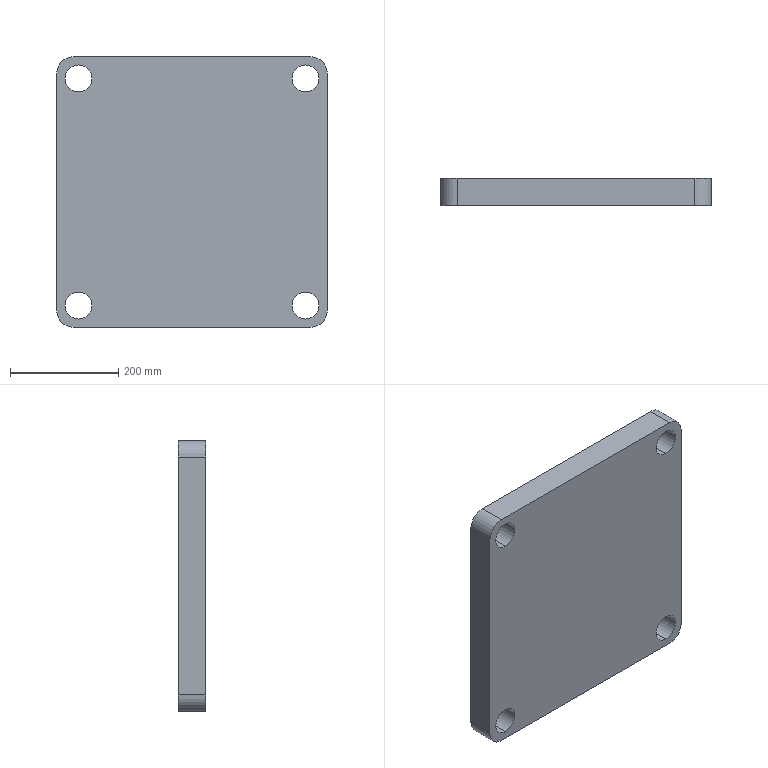Part | SolidWorks | features ICE 2, Extrusion 1 | 1 solid | 27 faces | box 500 x 50 x 500 mm | volume 6892126 mm3 | cylinder 16 | plane 11 | commonest cylinder face diameters 50 x8 60 x4 70 x4
STEP:
#1=CARTESIAN_POINT('',(-210.,0.,185.));
#2=VERTEX_POINT('',#1);
#3=CARTESIAN_POINT('',(-210.,0.,235.));
#4=VERTEX_POINT('',#3);
#5=CARTESIAN_POINT('',(-210.,0.,210.));
#6=DIRECTION('',(0.,1.,0.));
#7=DIRECTION('',(0.,0.,-1.));
#8=AXIS2_PLACEMENT_3D('',#5,#6,#7);
#9=CIRCLE('',#8,25.);
#10=EDGE_CURVE('',#2,#4,#9,.T.);
#11=ORIENTED_EDGE('',*,*,#10,.F.);
#12=CARTESIAN_POINT('',(-210.,50.,185.));
#13=VERTEX_POINT('',#12);
#14=CARTESIAN_POINT('',(-210.,-0.001,185.));
#15=DIRECTION('',(0.,1.,0.));
#16=VECTOR('',#15,1000.);
#17=LINE('',#14,#16);
#18=EDGE_CURVE('',#2,#13,#17,.T.);
#19=ORIENTED_EDGE('',*,*,#18,.T.);
#20=CARTESIAN_POINT('',(-210.,50.,235.));
#21=VERTEX_POINT('',#20);
#22=CARTESIAN_POINT('',(-210.,50.,210.));
#23=DIRECTION('',(0.,1.,0.));
#24=DIRECTION('',(0.,0.,-1.));
#25=AXIS2_PLACEMENT_3D('',#22,#23,#24);
#26=CIRCLE('',#25,25.);
#27=EDGE_CURVE('',#13,#21,#26,.T.);
#28=ORIENTED_EDGE('',*,*,#27,.T.);
#29=CARTESIAN_POINT('',(-210.,-0.001,235.));
#30=DIRECTION('',(0.,1.,0.));
#31=VECTOR('',#30,1000.);
#32=LINE('',#29,#31);
#33=EDGE_CURVE('',#4,#21,#32,.T.);
#34=ORIENTED_EDGE('',*,*,#33,.F.);
#35=EDGE_LOOP('',(#11,#19,#28,#34));
#36=FACE_OUTER_BOUND('',#35,.T.);
#37=CARTESIAN_POINT('',(-210.,-0.001,210.));
#38=DIRECTION('',(0.,1.,0.));
#39=DIRECTION('',(0.,0.,1.));
#40=AXIS2_PLACEMENT_3D('',#37,#38,#39);
#41=CYLINDRICAL_SURFACE('',#40,25.);
#42=ADVANCED_FACE('',(#36),#41,.F.);
#43=CARTESIAN_POINT('',(210.,0.,185.));
#44=VERTEX_POINT('',#43);
#45=CARTESIAN_POINT('',(210.,0.,235.));
#46=VERTEX_POINT('',#45);
#47=CARTESIAN_POINT('',(210.,0.,210.));
#48=DIRECTION('',(0.,1.,0.));
#49=DIRECTION('',(0.,0.,-1.));
#50=AXIS2_PLACEMENT_3D('',#47,#48,#49);
#51=CIRCLE('',#50,25.);
#52=EDGE_CURVE('',#44,#46,#51,.T.);
#53=ORIENTED_EDGE('',*,*,#52,.F.);
#54=CARTESIAN_POINT('',(210.,50.,185.));
#55=VERTEX_POINT('',#54);
#56=CARTESIAN_POINT('',(210.,-0.001,185.));
#57=DIRECTION('',(0.,1.,0.));
#58=VECTOR('',#57,1000.);
#59=LINE('',#56,#58);
#60=EDGE_CURVE('',#44,#55,#59,.T.);
#61=ORIENTED_EDGE('',*,*,#60,.T.);
#62=CARTESIAN_POINT('',(210.,50.,235.));
#63=VERTEX_POINT('',#62);
#64=CARTESIAN_POINT('',(210.,50.,210.));
#65=DIRECTION('',(0.,1.,0.));
#66=DIRECTION('',(0.,0.,1.));
#67=AXIS2_PLACEMENT_3D('',#64,#65,#66);
#68=CIRCLE('',#67,25.);
#69=EDGE_CURVE('',#55,#63,#68,.T.);
#70=ORIENTED_EDGE('',*,*,#69,.T.);
#71=CARTESIAN_POINT('',(210.,-0.001,235.));
#72=DIRECTION('',(0.,1.,0.));
#73=VECTOR('',#72,1000.);
#74=LINE('',#71,#73);
#75=EDGE_CURVE('',#46,#63,#74,.T.);
#76=ORIENTED_EDGE('',*,*,#75,.F.);
#77=EDGE_LOOP('',(#53,#61,#70,#76));
#78=FACE_OUTER_BOUND('',#77,.T.);
#79=CARTESIAN_POINT('',(210.,-0.001,210.));
#80=DIRECTION('',(0.,1.,0.));
#81=DIRECTION('',(0.,0.,1.));
#82=AXIS2_PLACEMENT_3D('',#79,#80,#81);
#83=CYLINDRICAL_SURFACE('',#82,25.);
#84=ADVANCED_FACE('',(#78),#83,.F.);
#85=CARTESIAN_POINT('',(210.,0.,-235.));
#86=VERTEX_POINT('',#85);
#87=CARTESIAN_POINT('',(210.,0.,-185.));
#88=VERTEX_POINT('',#87);
#89=CARTESIAN_POINT('',(210.,0.,-210.));
#90=DIRECTION('',(0.,1.,0.));
#91=DIRECTION('',(0.,0.,-1.));
#92=AXIS2_PLACEMENT_3D('',#89,#90,#91);
#93=CIRCLE('',#92,25.);
#94=EDGE_CURVE('',#86,#88,#93,.T.);
#95=ORIENTED_EDGE('',*,*,#94,.F.);
#96=CARTESIAN_POINT('',(210.,50.,-235.));
#97=VERTEX_POINT('',#96);
#98=CARTESIAN_POINT('',(210.,-0.001,-235.));
#99=DIRECTION('',(0.,1.,0.));
#100=VECTOR('',#99,1000.);
#101=LINE('',#98,#100);
#102=EDGE_CURVE('',#86,#97,#101,.T.);
#103=ORIENTED_EDGE('',*,*,#102,.T.);
#104=CARTESIAN_POINT('',(210.,50.,-185.));
#105=VERTEX_POINT('',#104);
#106=CARTESIAN_POINT('',(210.,50.,-210.));
#107=DIRECTION('',(0.,1.,0.));
#108=DIRECTION('',(0.,0.,-1.));
#109=AXIS2_PLACEMENT_3D('',#106,#107,#108);
#110=CIRCLE('',#109,25.);
#111=EDGE_CURVE('',#97,#105,#110,.T.);
#112=ORIENTED_EDGE('',*,*,#111,.T.);
#113=CARTESIAN_POINT('',(210.,-0.001,-185.));
#114=DIRECTION('',(0.,1.,0.));
#115=VECTOR('',#114,1000.);
#116=LINE('',#113,#115);
#117=EDGE_CURVE('',#88,#105,#116,.T.);
#118=ORIENTED_EDGE('',*,*,#117,.F.);
#119=EDGE_LOOP('',(#95,#103,#112,#118));
#120=FACE_OUTER_BOUND('',#119,.T.);
#121=CARTESIAN_POINT('',(210.,-0.001,-210.));
#122=DIRECTION('',(0.,1.,0.));
#123=DIRECTION('',(0.,0.,1.));
#124=AXIS2_PLACEMENT_3D('',#121,#122,#123);
#125=CYLINDRICAL_SURFACE('',#124,25.);
#126=ADVANCED_FACE('',(#120),#125,.F.);
#127=CARTESIAN_POINT('',(-210.,0.,-235.));
#128=VERTEX_POINT('',#127);
#129=CARTESIAN_POINT('',(-210.,0.,-185.));
#130=VERTEX_POINT('',#129);
#131=CARTESIAN_POINT('',(-210.,0.,-210.));
#132=DIRECTION('',(0.,1.,0.));
#133=DIRECTION('',(0.,0.,-1.));
#134=AXIS2_PLACEMENT_3D('',#131,#132,#133);
#135=CIRCLE('',#134,25.);
#136=EDGE_CURVE('',#128,#130,#135,.T.);
#137=ORIENTED_EDGE('',*,*,#136,.F.);
#138=CARTESIAN_POINT('',(-210.,50.,-235.));
#139=VERTEX_POINT('',#138);
#140=CARTESIAN_POINT('',(-210.,-0.001,-235.));
#141=DIRECTION('',(0.,1.,0.));
#142=VECTOR('',#141,1000.);
#143=LINE('',#140,#142);
#144=EDGE_CURVE('',#128,#139,#143,.T.);
#145=ORIENTED_EDGE('',*,*,#144,.T.);
#146=CARTESIAN_POINT('',(-210.,50.,-185.));
#147=VERTEX_POINT('',#146);
#148=CARTESIAN_POINT('',(-210.,50.,-210.));
#149=DIRECTION('',(0.,1.,0.));
#150=DIRECTION('',(0.,0.,1.));
#151=AXIS2_PLACEMENT_3D('',#148,#149,#150);
#152=CIRCLE('',#151,25.);
#153=EDGE_CURVE('',#139,#147,#152,.T.);
#154=ORIENTED_EDGE('',*,*,#153,.T.);
#155=CARTESIAN_POINT('',(-210.,-0.001,-185.));
#156=DIRECTION('',(0.,1.,0.));
#157=VECTOR('',#156,1000.);
#158=LINE('',#155,#157);
#159=EDGE_CURVE('',#130,#147,#158,.T.);
#160=ORIENTED_EDGE('',*,*,#159,.F.);
#161=EDGE_LOOP('',(#137,#145,#154,#160));
#162=FACE_OUTER_BOUND('',#161,.T.);
#163=CARTESIAN_POINT('',(-210.,-0.001,-210.));
#164=DIRECTION('',(0.,1.,0.));
#165=DIRECTION('',(0.,0.,1.));
#166=AXIS2_PLACEMENT_3D('',#163,#164,#165);
#167=CYLINDRICAL_SURFACE('',#166,25.);
#168=ADVANCED_FACE('',(#162),#167,.F.);
#169=CARTESIAN_POINT('',(-250.,0.,220.));
#170=VERTEX_POINT('',#169);
#171=CARTESIAN_POINT('',(-220.,0.,250.));
#172=VERTEX_POINT('',#171);
#173=CARTESIAN_POINT('',(-220.,0.,220.));
#174=DIRECTION('',(0.,1.,0.));
#175=DIRECTION('',(0.,0.,-1.));
#176=AXIS2_PLACEMENT_3D('',#173,#174,#175);
#177=CIRCLE('',#176,30.);
#178=EDGE_CURVE('',#170,#172,#177,.T.);
#179=ORIENTED_EDGE('',*,*,#178,.T.);
#180=CARTESIAN_POINT('',(-220.,50.,250.));
#181=VERTEX_POINT('',#180);
#182=CARTESIAN_POINT('',(-220.,50.,250.));
#183=DIRECTION('',(0.,-1.,0.));
#184=VECTOR('',#183,1000.);
#185=LINE('',#182,#184);
#186=EDGE_CURVE('',#181,#172,#185,.T.);
#187=ORIENTED_EDGE('',*,*,#186,.F.);
#188=CARTESIAN_POINT('',(-250.,50.,220.));
#189=VERTEX_POINT('',#188);
#190=CARTESIAN_POINT('',(-220.,50.,220.));
#191=DIRECTION('',(0.,1.,0.));
#192=DIRECTION('',(0.,0.,-1.));
#193=AXIS2_PLACEMENT_3D('',#190,#191,#192);
#194=CIRCLE('',#193,30.);
#195=EDGE_CURVE('',#189,#181,#194,.T.);
#196=ORIENTED_EDGE('',*,*,#195,.F.);
#197=CARTESIAN_POINT('',(-250.,50.,220.));
#198=DIRECTION('',(0.,-1.,0.));
#199=VECTOR('',#198,1000.);
#200=LINE('',#197,#199);
#201=EDGE_CURVE('',#189,#170,#200,.T.);
#202=ORIENTED_EDGE('',*,*,#201,.T.);
#203=EDGE_LOOP('',(#179,#187,#196,#202));
#204=FACE_OUTER_BOUND('',#203,.T.);
#205=CARTESIAN_POINT('',(-220.,50.,220.));
#206=DIRECTION('',(0.,-1.,0.));
#207=DIRECTION('',(0.,0.,-1.));
#208=AXIS2_PLACEMENT_3D('',#205,#206,#207);
#209=CYLINDRICAL_SURFACE('',#208,30.);
#210=ADVANCED_FACE('',(#204),#209,.T.);
#211=CARTESIAN_POINT('',(220.,0.,250.));
#212=VERTEX_POINT('',#211);
#213=CARTESIAN_POINT('',(-220.,0.,250.));
#214=DIRECTION('',(1.,0.,0.));
#215=VECTOR('',#214,1000.);
#216=LINE('',#213,#215);
#217=EDGE_CURVE('',#172,#212,#216,.T.);
#218=ORIENTED_EDGE('',*,*,#217,.T.);
#219=CARTESIAN_POINT('',(220.,50.,250.));
#220=VERTEX_POINT('',#219);
#221=CARTESIAN_POINT('',(220.,50.,250.));
#222=DIRECTION('',(0.,-1.,0.));
#223=VECTOR('',#222,1000.);
#224=LINE('',#221,#223);
#225=EDGE_CURVE('',#220,#212,#224,.T.);
#226=ORIENTED_EDGE('',*,*,#225,.F.);
#227=CARTESIAN_POINT('',(-220.,50.,250.));
#228=DIRECTION('',(1.,0.,0.));
#229=VECTOR('',#228,1000.);
#230=LINE('',#227,#229);
#231=EDGE_CURVE('',#181,#220,#230,.T.);
#232=ORIENTED_EDGE('',*,*,#231,.F.);
#233=ORIENTED_EDGE('',*,*,#186,.T.);
#234=EDGE_LOOP('',(#218,#226,#232,#233));
#235=FACE_OUTER_BOUND('',#234,.T.);
#236=CARTESIAN_POINT('',(-220.,50.,250.));
#237=DIRECTION('',(0.,0.,-1.));
#238=DIRECTION('',(-1.,0.,0.));
#239=AXIS2_PLACEMENT_3D('',#236,#237,#238);
#240=PLANE('',#239);
#241=ADVANCED_FACE('',(#235),#240,.F.);
#242=CARTESIAN_POINT('',(250.,0.,220.));
#243=VERTEX_POINT('',#242);
#244=CARTESIAN_POINT('',(220.,0.,220.));
#245=DIRECTION('',(0.,1.,0.));
#246=DIRECTION('',(0.,0.,1.));
#247=AXIS2_PLACEMENT_3D('',#244,#245,#246);
#248=CIRCLE('',#247,30.);
#249=EDGE_CURVE('',#212,#243,#248,.T.);
#250=ORIENTED_EDGE('',*,*,#249,.T.);
#251=CARTESIAN_POINT('',(250.,50.,220.));
#252=VERTEX_POINT('',#251);
#253=CARTESIAN_POINT('',(250.,50.,220.));
#254=DIRECTION('',(0.,-1.,0.));
#255=VECTOR('',#254,1000.);
#256=LINE('',#253,#255);
#257=EDGE_CURVE('',#252,#243,#256,.T.);
#258=ORIENTED_EDGE('',*,*,#257,.F.);
#259=CARTESIAN_POINT('',(220.,50.,220.));
#260=DIRECTION('',(0.,1.,0.));
#261=DIRECTION('',(0.,0.,1.));
#262=AXIS2_PLACEMENT_3D('',#259,#260,#261);
#263=CIRCLE('',#262,30.);
#264=EDGE_CURVE('',#220,#252,#263,.T.);
#265=ORIENTED_EDGE('',*,*,#264,.F.);
#266=ORIENTED_EDGE('',*,*,#225,.T.);
#267=EDGE_LOOP('',(#250,#258,#265,#266));
#268=FACE_OUTER_BOUND('',#267,.T.);
#269=CARTESIAN_POINT('',(220.,50.,220.));
#270=DIRECTION('',(0.,-1.,0.));
#271=DIRECTION('',(0.,0.,-1.));
#272=AXIS2_PLACEMENT_3D('',#269,#270,#271);
#273=CYLINDRICAL_SURFACE('',#272,30.);
#274=ADVANCED_FACE('',(#268),#273,.T.);
#275=CARTESIAN_POINT('',(250.,0.,-220.));
#276=VERTEX_POINT('',#275);
#277=CARTESIAN_POINT('',(250.,0.,220.));
#278=DIRECTION('',(0.,0.,-1.));
#279=VECTOR('',#278,1000.);
#280=LINE('',#277,#279);
#281=EDGE_CURVE('',#243,#276,#280,.T.);
#282=ORIENTED_EDGE('',*,*,#281,.T.);
#283=CARTESIAN_POINT('',(250.,50.,-220.));
#284=VERTEX_POINT('',#283);
#285=CARTESIAN_POINT('',(250.,50.,-220.));
#286=DIRECTION('',(0.,-1.,0.));
#287=VECTOR('',#286,1000.);
#288=LINE('',#285,#287);
#289=EDGE_CURVE('',#284,#276,#288,.T.);
#290=ORIENTED_EDGE('',*,*,#289,.F.);
#291=CARTESIAN_POINT('',(250.,50.,220.));
#292=DIRECTION('',(0.,0.,-1.));
#293=VECTOR('',#292,1000.);
#294=LINE('',#291,#293);
#295=EDGE_CURVE('',#252,#284,#294,.T.);
#296=ORIENTED_EDGE('',*,*,#295,.F.);
#297=ORIENTED_EDGE('',*,*,#257,.T.);
#298=EDGE_LOOP('',(#282,#290,#296,#297));
#299=FACE_OUTER_BOUND('',#298,.T.);
#300=CARTESIAN_POINT('',(250.,50.,220.));
#301=DIRECTION('',(-1.,0.,0.));
#302=DIRECTION('',(0.,0.,1.));
#303=AXIS2_PLACEMENT_3D('',#300,#301,#302);
#304=PLANE('',#303);
#305=ADVANCED_FACE('',(#299),#304,.F.);
#306=CARTESIAN_POINT('',(220.,0.,-250.));
#307=VERTEX_POINT('',#306);
#308=CARTESIAN_POINT('',(220.,0.,-220.));
#309=DIRECTION('',(0.,1.,0.));
#310=DIRECTION('',(0.,0.,1.));
#311=AXIS2_PLACEMENT_3D('',#308,#309,#310);
#312=CIRCLE('',#311,30.);
#313=EDGE_CURVE('',#276,#307,#312,.T.);
#314=ORIENTED_EDGE('',*,*,#313,.T.);
#315=CARTESIAN_POINT('',(220.,50.,-250.));
#316=VERTEX_POINT('',#315);
#317=CARTESIAN_POINT('',(220.,50.,-250.));
#318=DIRECTION('',(0.,-1.,0.));
#319=VECTOR('',#318,1000.);
#320=LINE('',#317,#319);
#321=EDGE_CURVE('',#316,#307,#320,.T.);
#322=ORIENTED_EDGE('',*,*,#321,.F.);
#323=CARTESIAN_POINT('',(220.,50.,-220.));
#324=DIRECTION('',(0.,1.,0.));
#325=DIRECTION('',(0.,0.,1.));
#326=AXIS2_PLACEMENT_3D('',#323,#324,#325);
#327=CIRCLE('',#326,30.);
#328=EDGE_CURVE('',#284,#316,#327,.T.);
#329=ORIENTED_EDGE('',*,*,#328,.F.);
#330=ORIENTED_EDGE('',*,*,#289,.T.);
#331=EDGE_LOOP('',(#314,#322,#329,#330));
#332=FACE_OUTER_BOUND('',#331,.T.);
#333=CARTESIAN_POINT('',(220.,50.,-220.));
#334=DIRECTION('',(0.,-1.,0.));
#335=DIRECTION('',(0.,0.,-1.));
#336=AXIS2_PLACEMENT_3D('',#333,#334,#335);
#337=CYLINDRICAL_SURFACE('',#336,30.);
#338=ADVANCED_FACE('',(#332),#337,.T.);
#339=CARTESIAN_POINT('',(-220.,0.,-250.));
#340=VERTEX_POINT('',#339);
#341=CARTESIAN_POINT('',(-220.,0.,-250.));
#342=DIRECTION('',(-1.,0.,0.));
#343=VECTOR('',#342,1000.);
#344=LINE('',#341,#343);
#345=EDGE_CURVE('',#307,#340,#344,.T.);
#346=ORIENTED_EDGE('',*,*,#345,.T.);
#347=CARTESIAN_POINT('',(-220.,50.,-250.));
#348=VERTEX_POINT('',#347);
#349=CARTESIAN_POINT('',(-220.,50.,-250.));
#350=DIRECTION('',(0.,-1.,0.));
#351=VECTOR('',#350,1000.);
#352=LINE('',#349,#351);
#353=EDGE_CURVE('',#348,#340,#352,.T.);
#354=ORIENTED_EDGE('',*,*,#353,.F.);
#355=CARTESIAN_POINT('',(-220.,50.,-250.));
#356=DIRECTION('',(-1.,0.,0.));
#357=VECTOR('',#356,1000.);
#358=LINE('',#355,#357);
#359=EDGE_CURVE('',#316,#348,#358,.T.);
#360=ORIENTED_EDGE('',*,*,#359,.F.);
#361=ORIENTED_EDGE('',*,*,#321,.T.);
#362=EDGE_LOOP('',(#346,#354,#360,#361));
#363=FACE_OUTER_BOUND('',#362,.T.);
#364=CARTESIAN_POINT('',(-220.,50.,-250.));
#365=DIRECTION('',(0.,0.,1.));
#366=DIRECTION('',(1.,0.,0.));
#367=AXIS2_PLACEMENT_3D('',#364,#365,#366);
#368=PLANE('',#367);
#369=ADVANCED_FACE('',(#363),#368,.F.);
#370=CARTESIAN_POINT('',(-250.,0.,-220.));
#371=VERTEX_POINT('',#370);
#372=CARTESIAN_POINT('',(-220.,0.,-220.));
#373=DIRECTION('',(0.,1.,0.));
#374=DIRECTION('',(0.,0.,-1.));
#375=AXIS2_PLACEMENT_3D('',#372,#373,#374);
#376=CIRCLE('',#375,30.);
#377=EDGE_CURVE('',#340,#371,#376,.T.);
#378=ORIENTED_EDGE('',*,*,#377,.T.);
#379=CARTESIAN_POINT('',(-250.,50.,-220.));
#380=VERTEX_POINT('',#379);
#381=CARTESIAN_POINT('',(-250.,50.,-220.));
#382=DIRECTION('',(0.,-1.,0.));
#383=VECTOR('',#382,1000.);
#384=LINE('',#381,#383);
#385=EDGE_CURVE('',#380,#371,#384,.T.);
#386=ORIENTED_EDGE('',*,*,#385,.F.);
#387=CARTESIAN_POINT('',(-220.,50.,-220.));
#388=DIRECTION('',(0.,1.,0.));
#389=DIRECTION('',(0.,0.,-1.));
#390=AXIS2_PLACEMENT_3D('',#387,#388,#389);
#391=CIRCLE('',#390,30.);
#392=EDGE_CURVE('',#348,#380,#391,.T.);
#393=ORIENTED_EDGE('',*,*,#392,.F.);
#394=ORIENTED_EDGE('',*,*,#353,.T.);
#395=EDGE_LOOP('',(#378,#386,#393,#394));
#396=FACE_OUTER_BOUND('',#395,.T.);
#397=CARTESIAN_POINT('',(-220.,50.,-220.));
#398=DIRECTION('',(0.,-1.,0.));
#399=DIRECTION('',(0.,0.,-1.));
#400=AXIS2_PLACEMENT_3D('',#397,#398,#399);
#401=CYLINDRICAL_SURFACE('',#400,30.);
#402=ADVANCED_FACE('',(#396),#401,.T.);
#403=CARTESIAN_POINT('',(-250.,0.,220.));
#404=DIRECTION('',(0.,0.,1.));
#405=VECTOR('',#404,1000.);
#406=LINE('',#403,#405);
#407=EDGE_CURVE('',#371,#170,#406,.T.);
#408=ORIENTED_EDGE('',*,*,#407,.T.);
#409=ORIENTED_EDGE('',*,*,#201,.F.);
#410=CARTESIAN_POINT('',(-250.,50.,220.));
#411=DIRECTION('',(0.,0.,1.));
#412=VECTOR('',#411,1000.);
#413=LINE('',#410,#412);
#414=EDGE_CURVE('',#380,#189,#413,.T.);
#415=ORIENTED_EDGE('',*,*,#414,.F.);
#416=ORIENTED_EDGE('',*,*,#385,.T.);
#417=EDGE_LOOP('',(#408,#409,#415,#416));
#418=FACE_OUTER_BOUND('',#417,.T.);
#419=CARTESIAN_POINT('',(-250.,50.,220.));
#420=DIRECTION('',(1.,0.,0.));
#421=DIRECTION('',(0.,0.,-1.));
#422=AXIS2_PLACEMENT_3D('',#419,#420,#421);
#423=PLANE('',#422);
#424=ADVANCED_FACE('',(#418),#423,.F.);
#425=CARTESIAN_POINT('',(-210.,50.,210.));
#426=DIRECTION('',(0.,1.,0.));
#427=DIRECTION('',(0.,0.,-1.));
#428=AXIS2_PLACEMENT_3D('',#425,#426,#427);
#429=CIRCLE('',#428,25.);
#430=EDGE_CURVE('',#21,#13,#429,.T.);
#431=ORIENTED_EDGE('',*,*,#430,.F.);
#432=ORIENTED_EDGE('',*,*,#27,.F.);
#433=EDGE_LOOP('',(#431,#432));
#434=FACE_BOUND('',#433,.T.);
#435=CARTESIAN_POINT('',(210.,50.,210.));
#436=DIRECTION('',(0.,1.,0.));
#437=DIRECTION('',(0.,0.,1.));
#438=AXIS2_PLACEMENT_3D('',#435,#436,#437);
#439=CIRCLE('',#438,25.);
#440=EDGE_CURVE('',#63,#55,#439,.T.);
#441=ORIENTED_EDGE('',*,*,#440,.F.);
#442=ORIENTED_EDGE('',*,*,#69,.F.);
#443=EDGE_LOOP('',(#441,#442));
#444=FACE_BOUND('',#443,.T.);
#445=CARTESIAN_POINT('',(210.,50.,-210.));
#446=DIRECTION('',(0.,1.,0.));
#447=DIRECTION('',(0.,0.,-1.));
#448=AXIS2_PLACEMENT_3D('',#445,#446,#447);
#449=CIRCLE('',#448,25.);
#450=EDGE_CURVE('',#105,#97,#449,.T.);
#451=ORIENTED_EDGE('',*,*,#450,.F.);
#452=ORIENTED_EDGE('',*,*,#111,.F.);
#453=EDGE_LOOP('',(#451,#452));
#454=FACE_BOUND('',#453,.T.);
#455=CARTESIAN_POINT('',(-210.,50.,-210.));
#456=DIRECTION('',(0.,1.,0.));
#457=DIRECTION('',(0.,0.,1.));
#458=AXIS2_PLACEMENT_3D('',#455,#456,#457);
#459=CIRCLE('',#458,25.);
#460=EDGE_CURVE('',#147,#139,#459,.T.);
#461=ORIENTED_EDGE('',*,*,#460,.F.);
#462=ORIENTED_EDGE('',*,*,#153,.F.);
#463=EDGE_LOOP('',(#461,#462));
#464=FACE_BOUND('',#463,.T.);
#465=CARTESIAN_POINT('',(210.,50.,175.));
#466=VERTEX_POINT('',#465);
#467=CARTESIAN_POINT('',(210.,50.,-175.));
#468=VERTEX_POINT('',#467);
#469=CARTESIAN_POINT('',(210.,50.,175.));
#470=DIRECTION('',(0.,0.,-1.));
#471=VECTOR('',#470,1000.);
#472=LINE('',#469,#471);
#473=EDGE_CURVE('',#466,#468,#472,.T.);
#474=ORIENTED_EDGE('',*,*,#473,.F.);
#475=CARTESIAN_POINT('',(175.,50.,210.));
#476=VERTEX_POINT('',#475);
#477=CARTESIAN_POINT('',(210.,50.,210.));
#478=DIRECTION('',(0.,-1.,0.));
#479=DIRECTION('',(0.,0.,-1.));
#480=AXIS2_PLACEMENT_3D('',#477,#478,#479);
#481=CIRCLE('',#480,35.);
#482=EDGE_CURVE('',#476,#466,#481,.T.);
#483=ORIENTED_EDGE('',*,*,#482,.F.);
#484=CARTESIAN_POINT('',(-175.,50.,210.));
#485=VERTEX_POINT('',#484);
#486=CARTESIAN_POINT('',(-175.,50.,210.));
#487=DIRECTION('',(1.,0.,0.));
#488=VECTOR('',#487,1000.);
#489=LINE('',#486,#488);
#490=EDGE_CURVE('',#485,#476,#489,.T.);
#491=ORIENTED_EDGE('',*,*,#490,.F.);
#492=CARTESIAN_POINT('',(-210.,50.,175.));
#493=VERTEX_POINT('',#492);
#494=CARTESIAN_POINT('',(-210.,50.,210.));
#495=DIRECTION('',(0.,-1.,0.));
#496=DIRECTION('',(0.,0.,1.));
#497=AXIS2_PLACEMENT_3D('',#494,#495,#496);
#498=CIRCLE('',#497,35.);
#499=EDGE_CURVE('',#493,#485,#498,.T.);
#500=ORIENTED_EDGE('',*,*,#499,.F.);
#501=CARTESIAN_POINT('',(-210.,50.,-175.));
#502=VERTEX_POINT('',#501);
#503=CARTESIAN_POINT('',(-210.,50.,175.));
#504=DIRECTION('',(0.,0.,1.));
#505=VECTOR('',#504,1000.);
#506=LINE('',#503,#505);
#507=EDGE_CURVE('',#502,#493,#506,.T.);
#508=ORIENTED_EDGE('',*,*,#507,.F.);
#509=CARTESIAN_POINT('',(-175.,50.,-210.));
#510=VERTEX_POINT('',#509);
#511=CARTESIAN_POINT('',(-210.,50.,-210.));
#512=DIRECTION('',(0.,-1.,0.));
#513=DIRECTION('',(0.,0.,-1.));
#514=AXIS2_PLACEMENT_3D('',#511,#512,#513);
#515=CIRCLE('',#514,35.);
#516=EDGE_CURVE('',#510,#502,#515,.T.);
#517=ORIENTED_EDGE('',*,*,#516,.F.);
#518=CARTESIAN_POINT('',(175.,50.,-210.));
#519=VERTEX_POINT('',#518);
#520=CARTESIAN_POINT('',(-175.,50.,-210.));
#521=DIRECTION('',(-1.,0.,0.));
#522=VECTOR('',#521,1000.);
#523=LINE('',#520,#522);
#524=EDGE_CURVE('',#519,#510,#523,.T.);
#525=ORIENTED_EDGE('',*,*,#524,.F.);
#526=CARTESIAN_POINT('',(210.,50.,-210.));
#527=DIRECTION('',(0.,-1.,0.));
#528=DIRECTION('',(0.,0.,1.));
#529=AXIS2_PLACEMENT_3D('',#526,#527,#528);
#530=CIRCLE('',#529,35.);
#531=EDGE_CURVE('',#468,#519,#530,.T.);
#532=ORIENTED_EDGE('',*,*,#531,.F.);
#533=EDGE_LOOP('',(#474,#483,#491,#500,#508,#517,#525,#532));
#534=FACE_BOUND('',#533,.T.);
#535=ORIENTED_EDGE('',*,*,#195,.T.);
#536=ORIENTED_EDGE('',*,*,#231,.T.);
#537=ORIENTED_EDGE('',*,*,#264,.T.);
#538=ORIENTED_EDGE('',*,*,#295,.T.);
#539=ORIENTED_EDGE('',*,*,#328,.T.);
#540=ORIENTED_EDGE('',*,*,#359,.T.);
#541=ORIENTED_EDGE('',*,*,#392,.T.);
#542=ORIENTED_EDGE('',*,*,#414,.T.);
#543=EDGE_LOOP('',(#535,#536,#537,#538,#539,#540,#541,#542));
#544=FACE_OUTER_BOUND('',#543,.T.);
#545=CARTESIAN_POINT('',(-220.,50.,220.));
#546=DIRECTION('',(0.,-1.,0.));
#547=DIRECTION('',(0.,0.,-1.));
#548=AXIS2_PLACEMENT_3D('',#545,#546,#547);
#549=PLANE('',#548);
#550=ADVANCED_FACE('',(#434,#444,#454,#464,#534,#544),#549,.F.);
#551=CARTESIAN_POINT('',(-210.,0.,210.));
#552=DIRECTION('',(0.,1.,0.));
#553=DIRECTION('',(0.,0.,-1.));
#554=AXIS2_PLACEMENT_3D('',#551,#552,#553);
#555=CIRCLE('',#554,25.);
#556=EDGE_CURVE('',#4,#2,#555,.T.);
#557=ORIENTED_EDGE('',*,*,#556,.T.);
#558=ORIENTED_EDGE('',*,*,#10,.T.);
#559=EDGE_LOOP('',(#557,#558));
#560=FACE_BOUND('',#559,.T.);
#561=CARTESIAN_POINT('',(210.,0.,210.));
#562=DIRECTION('',(0.,1.,0.));
#563=DIRECTION('',(0.,0.,-1.));
#564=AXIS2_PLACEMENT_3D('',#561,#562,#563);
#565=CIRCLE('',#564,25.);
#566=EDGE_CURVE('',#46,#44,#565,.T.);
#567=ORIENTED_EDGE('',*,*,#566,.T.);
#568=ORIENTED_EDGE('',*,*,#52,.T.);
#569=EDGE_LOOP('',(#567,#568));
#570=FACE_BOUND('',#569,.T.);
#571=CARTESIAN_POINT('',(210.,0.,-210.));
#572=DIRECTION('',(0.,1.,0.));
#573=DIRECTION('',(0.,0.,-1.));
#574=AXIS2_PLACEMENT_3D('',#571,#572,#573);
#575=CIRCLE('',#574,25.);
#576=EDGE_CURVE('',#88,#86,#575,.T.);
#577=ORIENTED_EDGE('',*,*,#576,.T.);
#578=ORIENTED_EDGE('',*,*,#94,.T.);
#579=EDGE_LOOP('',(#577,#578));
#580=FACE_BOUND('',#579,.T.);
#581=CARTESIAN_POINT('',(-210.,0.,-210.));
#582=DIRECTION('',(0.,1.,0.));
#583=DIRECTION('',(0.,0.,-1.));
#584=AXIS2_PLACEMENT_3D('',#581,#582,#583);
#585=CIRCLE('',#584,25.);
#586=EDGE_CURVE('',#130,#128,#585,.T.);
#587=ORIENTED_EDGE('',*,*,#586,.T.);
#588=ORIENTED_EDGE('',*,*,#136,.T.);
#589=EDGE_LOOP('',(#587,#588));
#590=FACE_BOUND('',#589,.T.);
#591=ORIENTED_EDGE('',*,*,#178,.F.);
#592=ORIENTED_EDGE('',*,*,#407,.F.);
#593=ORIENTED_EDGE('',*,*,#377,.F.);
#594=ORIENTED_EDGE('',*,*,#345,.F.);
#595=ORIENTED_EDGE('',*,*,#313,.F.);
#596=ORIENTED_EDGE('',*,*,#281,.F.);
#597=ORIENTED_EDGE('',*,*,#249,.F.);
#598=ORIENTED_EDGE('',*,*,#217,.F.);
#599=EDGE_LOOP('',(#591,#592,#593,#594,#595,#596,#597,#598));
#600=FACE_OUTER_BOUND('',#599,.T.);
#601=CARTESIAN_POINT('',(-220.,0.,220.));
#602=DIRECTION('',(0.,-1.,0.));
#603=DIRECTION('',(0.,0.,-1.));
#604=AXIS2_PLACEMENT_3D('',#601,#602,#603);
#605=PLANE('',#604);
#606=ADVANCED_FACE('',(#560,#570,#580,#590,#600),#605,.T.);
#607=ORIENTED_EDGE('',*,*,#482,.T.);
#608=CARTESIAN_POINT('',(210.,20.,175.));
#609=VERTEX_POINT('',#608);
#610=CARTESIAN_POINT('',(210.,20.,175.));
#611=DIRECTION('',(0.,1.,0.));
#612=VECTOR('',#611,1000.);
#613=LINE('',#610,#612);
#614=EDGE_CURVE('',#609,#466,#613,.T.);
#615=ORIENTED_EDGE('',*,*,#614,.F.);
#616=CARTESIAN_POINT('',(175.,20.,210.));
#617=VERTEX_POINT('',#616);
#618=CARTESIAN_POINT('',(210.,20.,210.));
#619=DIRECTION('',(0.,-1.,0.));
#620=DIRECTION('',(0.,0.,-1.));
#621=AXIS2_PLACEMENT_3D('',#618,#619,#620);
#622=CIRCLE('',#621,35.);
#623=EDGE_CURVE('',#617,#609,#622,.T.);
#624=ORIENTED_EDGE('',*,*,#623,.F.);
#625=CARTESIAN_POINT('',(175.,20.,210.));
#626=DIRECTION('',(0.,1.,0.));
#627=VECTOR('',#626,1000.);
#628=LINE('',#625,#627);
#629=EDGE_CURVE('',#617,#476,#628,.T.);
#630=ORIENTED_EDGE('',*,*,#629,.T.);
#631=EDGE_LOOP('',(#607,#615,#624,#630));
#632=FACE_OUTER_BOUND('',#631,.T.);
#633=CARTESIAN_POINT('',(210.,20.,210.));
#634=DIRECTION('',(0.,1.,0.));
#635=DIRECTION('',(0.,0.,1.));
#636=AXIS2_PLACEMENT_3D('',#633,#634,#635);
#637=CYLINDRICAL_SURFACE('',#636,35.);
#638=ADVANCED_FACE('',(#632),#637,.T.);
#639=ORIENTED_EDGE('',*,*,#490,.T.);
#640=ORIENTED_EDGE('',*,*,#629,.F.);
#641=CARTESIAN_POINT('',(-175.,20.,210.));
#642=VERTEX_POINT('',#641);
#643=CARTESIAN_POINT('',(-175.,20.,210.));
#644=DIRECTION('',(1.,0.,0.));
#645=VECTOR('',#644,1000.);
#646=LINE('',#643,#645);
#647=EDGE_CURVE('',#642,#617,#646,.T.);
#648=ORIENTED_EDGE('',*,*,#647,.F.);
#649=CARTESIAN_POINT('',(-175.,20.,210.));
#650=DIRECTION('',(0.,1.,0.));
#651=VECTOR('',#650,1000.);
#652=LINE('',#649,#651);
#653=EDGE_CURVE('',#642,#485,#652,.T.);
#654=ORIENTED_EDGE('',*,*,#653,.T.);
#655=EDGE_LOOP('',(#639,#640,#648,#654));
#656=FACE_OUTER_BOUND('',#655,.T.);
#657=CARTESIAN_POINT('',(-175.,20.,210.));
#658=DIRECTION('',(0.,0.,1.));
#659=DIRECTION('',(1.,0.,0.));
#660=AXIS2_PLACEMENT_3D('',#657,#658,#659);
#661=PLANE('',#660);
#662=ADVANCED_FACE('',(#656),#661,.F.);
#663=ORIENTED_EDGE('',*,*,#499,.T.);
#664=ORIENTED_EDGE('',*,*,#653,.F.);
#665=CARTESIAN_POINT('',(-210.,20.,175.));
#666=VERTEX_POINT('',#665);
#667=CARTESIAN_POINT('',(-210.,20.,210.));
#668=DIRECTION('',(0.,-1.,0.));
#669=DIRECTION('',(0.,0.,1.));
#670=AXIS2_PLACEMENT_3D('',#667,#668,#669);
#671=CIRCLE('',#670,35.);
#672=EDGE_CURVE('',#666,#642,#671,.T.);
#673=ORIENTED_EDGE('',*,*,#672,.F.);
#674=CARTESIAN_POINT('',(-210.,20.,175.));
#675=DIRECTION('',(0.,1.,0.));
#676=VECTOR('',#675,1000.);
#677=LINE('',#674,#676);
#678=EDGE_CURVE('',#666,#493,#677,.T.);
#679=ORIENTED_EDGE('',*,*,#678,.T.);
#680=EDGE_LOOP('',(#663,#664,#673,#679));
#681=FACE_OUTER_BOUND('',#680,.T.);
#682=CARTESIAN_POINT('',(-210.,20.,210.));
#683=DIRECTION('',(0.,1.,0.));
#684=DIRECTION('',(0.,0.,1.));
#685=AXIS2_PLACEMENT_3D('',#682,#683,#684);
#686=CYLINDRICAL_SURFACE('',#685,35.);
#687=ADVANCED_FACE('',(#681),#686,.T.);
#688=ORIENTED_EDGE('',*,*,#507,.T.);
#689=ORIENTED_EDGE('',*,*,#678,.F.);
#690=CARTESIAN_POINT('',(-210.,20.,-175.));
#691=VERTEX_POINT('',#690);
#692=CARTESIAN_POINT('',(-210.,20.,175.));
#693=DIRECTION('',(0.,0.,1.));
#694=VECTOR('',#693,1000.);
#695=LINE('',#692,#694);
#696=EDGE_CURVE('',#691,#666,#695,.T.);
#697=ORIENTED_EDGE('',*,*,#696,.F.);
#698=CARTESIAN_POINT('',(-210.,20.,-175.));
#699=DIRECTION('',(0.,1.,0.));
#700=VECTOR('',#699,1000.);
#701=LINE('',#698,#700);
#702=EDGE_CURVE('',#691,#502,#701,.T.);
#703=ORIENTED_EDGE('',*,*,#702,.T.);
#704=EDGE_LOOP('',(#688,#689,#697,#703));
#705=FACE_OUTER_BOUND('',#704,.T.);
#706=CARTESIAN_POINT('',(-210.,20.,175.));
#707=DIRECTION('',(-1.,0.,0.));
#708=DIRECTION('',(0.,0.,1.));
#709=AXIS2_PLACEMENT_3D('',#706,#707,#708);
#710=PLANE('',#709);
#711=ADVANCED_FACE('',(#705),#710,.F.);
#712=ORIENTED_EDGE('',*,*,#516,.T.);
#713=ORIENTED_EDGE('',*,*,#702,.F.);
#714=CARTESIAN_POINT('',(-175.,20.,-210.));
#715=VERTEX_POINT('',#714);
#716=CARTESIAN_POINT('',(-210.,20.,-210.));
#717=DIRECTION('',(0.,-1.,0.));
#718=DIRECTION('',(0.,0.,-1.));
#719=AXIS2_PLACEMENT_3D('',#716,#717,#718);
#720=CIRCLE('',#719,35.);
#721=EDGE_CURVE('',#715,#691,#720,.T.);
#722=ORIENTED_EDGE('',*,*,#721,.F.);
#723=CARTESIAN_POINT('',(-175.,20.,-210.));
#724=DIRECTION('',(0.,1.,0.));
#725=VECTOR('',#724,1000.);
#726=LINE('',#723,#725);
#727=EDGE_CURVE('',#715,#510,#726,.T.);
#728=ORIENTED_EDGE('',*,*,#727,.T.);
#729=EDGE_LOOP('',(#712,#713,#722,#728));
#730=FACE_OUTER_BOUND('',#729,.T.);
#731=CARTESIAN_POINT('',(-210.,20.,-210.));
#732=DIRECTION('',(0.,1.,0.));
#733=DIRECTION('',(0.,0.,1.));
#734=AXIS2_PLACEMENT_3D('',#731,#732,#733);
#735=CYLINDRICAL_SURFACE('',#734,35.);
#736=ADVANCED_FACE('',(#730),#735,.T.);
#737=ORIENTED_EDGE('',*,*,#524,.T.);
#738=ORIENTED_EDGE('',*,*,#727,.F.);
#739=CARTESIAN_POINT('',(175.,20.,-210.));
#740=VERTEX_POINT('',#739);
#741=CARTESIAN_POINT('',(-175.,20.,-210.));
#742=DIRECTION('',(-1.,0.,0.));
#743=VECTOR('',#742,1000.);
#744=LINE('',#741,#743);
#745=EDGE_CURVE('',#740,#715,#744,.T.);
#746=ORIENTED_EDGE('',*,*,#745,.F.);
#747=CARTESIAN_POINT('',(175.,20.,-210.));
#748=DIRECTION('',(0.,1.,0.));
#749=VECTOR('',#748,1000.);
#750=LINE('',#747,#749);
#751=EDGE_CURVE('',#740,#519,#750,.T.);
#752=ORIENTED_EDGE('',*,*,#751,.T.);
#753=EDGE_LOOP('',(#737,#738,#746,#752));
#754=FACE_OUTER_BOUND('',#753,.T.);
#755=CARTESIAN_POINT('',(-175.,20.,-210.));
#756=DIRECTION('',(0.,0.,-1.));
#757=DIRECTION('',(-1.,0.,0.));
#758=AXIS2_PLACEMENT_3D('',#755,#756,#757);
#759=PLANE('',#758);
#760=ADVANCED_FACE('',(#754),#759,.F.);
#761=ORIENTED_EDGE('',*,*,#531,.T.);
#762=ORIENTED_EDGE('',*,*,#751,.F.);
#763=CARTESIAN_POINT('',(210.,20.,-175.));
#764=VERTEX_POINT('',#763);
#765=CARTESIAN_POINT('',(210.,20.,-210.));
#766=DIRECTION('',(0.,-1.,0.));
#767=DIRECTION('',(0.,0.,1.));
#768=AXIS2_PLACEMENT_3D('',#765,#766,#767);
#769=CIRCLE('',#768,35.);
#770=EDGE_CURVE('',#764,#740,#769,.T.);
#771=ORIENTED_EDGE('',*,*,#770,.F.);
#772=CARTESIAN_POINT('',(210.,20.,-175.));
#773=DIRECTION('',(0.,1.,0.));
#774=VECTOR('',#773,1000.);
#775=LINE('',#772,#774);
#776=EDGE_CURVE('',#764,#468,#775,.T.);
#777=ORIENTED_EDGE('',*,*,#776,.T.);
#778=EDGE_LOOP('',(#761,#762,#771,#777));
#779=FACE_OUTER_BOUND('',#778,.T.);
#780=CARTESIAN_POINT('',(210.,20.,-210.));
#781=DIRECTION('',(0.,1.,0.));
#782=DIRECTION('',(0.,0.,1.));
#783=AXIS2_PLACEMENT_3D('',#780,#781,#782);
#784=CYLINDRICAL_SURFACE('',#783,35.);
#785=ADVANCED_FACE('',(#779),#784,.T.);
#786=ORIENTED_EDGE('',*,*,#473,.T.);
#787=ORIENTED_EDGE('',*,*,#776,.F.);
#788=CARTESIAN_POINT('',(210.,20.,175.));
#789=DIRECTION('',(0.,0.,-1.));
#790=VECTOR('',#789,1000.);
#791=LINE('',#788,#790);
#792=EDGE_CURVE('',#609,#764,#791,.T.);
#793=ORIENTED_EDGE('',*,*,#792,.F.);
#794=ORIENTED_EDGE('',*,*,#614,.T.);
#795=EDGE_LOOP('',(#786,#787,#793,#794));
#796=FACE_OUTER_BOUND('',#795,.T.);
#797=CARTESIAN_POINT('',(210.,20.,175.));
#798=DIRECTION('',(1.,0.,0.));
#799=DIRECTION('',(0.,0.,-1.));
#800=AXIS2_PLACEMENT_3D('',#797,#798,#799);
#801=PLANE('',#800);
#802=ADVANCED_FACE('',(#796),#801,.F.);
#803=ORIENTED_EDGE('',*,*,#623,.T.);
#804=ORIENTED_EDGE('',*,*,#792,.T.);
#805=ORIENTED_EDGE('',*,*,#770,.T.);
#806=ORIENTED_EDGE('',*,*,#745,.T.);
#807=ORIENTED_EDGE('',*,*,#721,.T.);
#808=ORIENTED_EDGE('',*,*,#696,.T.);
#809=ORIENTED_EDGE('',*,*,#672,.T.);
#810=ORIENTED_EDGE('',*,*,#647,.T.);
#811=EDGE_LOOP('',(#803,#804,#805,#806,#807,#808,#809,#810));
#812=FACE_OUTER_BOUND('',#811,.T.);
#813=CARTESIAN_POINT('',(210.,20.,210.));
#814=DIRECTION('',(0.,-1.,0.));
#815=DIRECTION('',(0.,0.,-1.));
#816=AXIS2_PLACEMENT_3D('',#813,#814,#815);
#817=PLANE('',#816);
#818=ADVANCED_FACE('',(#812),#817,.F.);
#819=ORIENTED_EDGE('',*,*,#144,.F.);
#820=ORIENTED_EDGE('',*,*,#586,.F.);
#821=ORIENTED_EDGE('',*,*,#159,.T.);
#822=ORIENTED_EDGE('',*,*,#460,.T.);
#823=EDGE_LOOP('',(#819,#820,#821,#822));
#824=FACE_OUTER_BOUND('',#823,.T.);
#825=CARTESIAN_POINT('',(-210.,-0.001,-210.));
#826=DIRECTION('',(0.,1.,0.));
#827=DIRECTION('',(0.,0.,1.));
#828=AXIS2_PLACEMENT_3D('',#825,#826,#827);
#829=CYLINDRICAL_SURFACE('',#828,25.);
#830=ADVANCED_FACE('',(#824),#829,.F.);
#831=ORIENTED_EDGE('',*,*,#102,.F.);
#832=ORIENTED_EDGE('',*,*,#576,.F.);
#833=ORIENTED_EDGE('',*,*,#117,.T.);
#834=ORIENTED_EDGE('',*,*,#450,.T.);
#835=EDGE_LOOP('',(#831,#832,#833,#834));
#836=FACE_OUTER_BOUND('',#835,.T.);
#837=CARTESIAN_POINT('',(210.,-0.001,-210.));
#838=DIRECTION('',(0.,1.,0.));
#839=DIRECTION('',(0.,0.,1.));
#840=AXIS2_PLACEMENT_3D('',#837,#838,#839);
#841=CYLINDRICAL_SURFACE('',#840,25.);
#842=ADVANCED_FACE('',(#836),#841,.F.);
#843=ORIENTED_EDGE('',*,*,#60,.F.);
#844=ORIENTED_EDGE('',*,*,#566,.F.);
#845=ORIENTED_EDGE('',*,*,#75,.T.);
#846=ORIENTED_EDGE('',*,*,#440,.T.);
#847=EDGE_LOOP('',(#843,#844,#845,#846));
#848=FACE_OUTER_BOUND('',#847,.T.);
#849=CARTESIAN_POINT('',(210.,-0.001,210.));
#850=DIRECTION('',(0.,1.,0.));
#851=DIRECTION('',(0.,0.,1.));
#852=AXIS2_PLACEMENT_3D('',#849,#850,#851);
#853=CYLINDRICAL_SURFACE('',#852,25.);
#854=ADVANCED_FACE('',(#848),#853,.F.);
#855=ORIENTED_EDGE('',*,*,#18,.F.);
#856=ORIENTED_EDGE('',*,*,#556,.F.);
#857=ORIENTED_EDGE('',*,*,#33,.T.);
#858=ORIENTED_EDGE('',*,*,#430,.T.);
#859=EDGE_LOOP('',(#855,#856,#857,#858));
#860=FACE_OUTER_BOUND('',#859,.T.);
#861=CARTESIAN_POINT('',(-210.,-0.001,210.));
#862=DIRECTION('',(0.,1.,0.));
#863=DIRECTION('',(0.,0.,1.));
#864=AXIS2_PLACEMENT_3D('',#861,#862,#863);
#865=CYLINDRICAL_SURFACE('',#864,25.);
#866=ADVANCED_FACE('',(#860),#865,.F.);
#867=CLOSED_SHELL('',(#42,#84,#126,#168,#210,#241,#274,#305,#338,#369,#402,#424,#550,#606,#638,#662,#687,#711,#736,#760,#785,#802,#818,#830,#842,#854,#866));
#868=MANIFOLD_SOLID_BREP('',#867);
#869=CARTESIAN_POINT('',(0.,0.,0.));
#870=DIRECTION('',(0.,0.,1.));
#871=DIRECTION('',(1.,0.,0.));
#872=AXIS2_PLACEMENT_3D('',#869,#870,#871);
#873=(LENGTH_UNIT()NAMED_UNIT(*)SI_UNIT(.MILLI.,.METRE.));
#874=UNCERTAINTY_MEASURE_WITH_UNIT(LENGTH_MEASURE(0.00001),#873,'','');
#875=(NAMED_UNIT(*)PLANE_ANGLE_UNIT()SI_UNIT($,.RADIAN.));
#876=(NAMED_UNIT(*)SI_UNIT($,.STERADIAN.)SOLID_ANGLE_UNIT());
#877=(GEOMETRIC_REPRESENTATION_CONTEXT(3)GLOBAL_UNCERTAINTY_ASSIGNED_CONTEXT((#874))GLOBAL_UNIT_ASSIGNED_CONTEXT((#873,#875,#876))REPRESENTATION_CONTEXT('',''));
#878=ADVANCED_BREP_SHAPE_REPRESENTATION('',(#868,#872),#877);